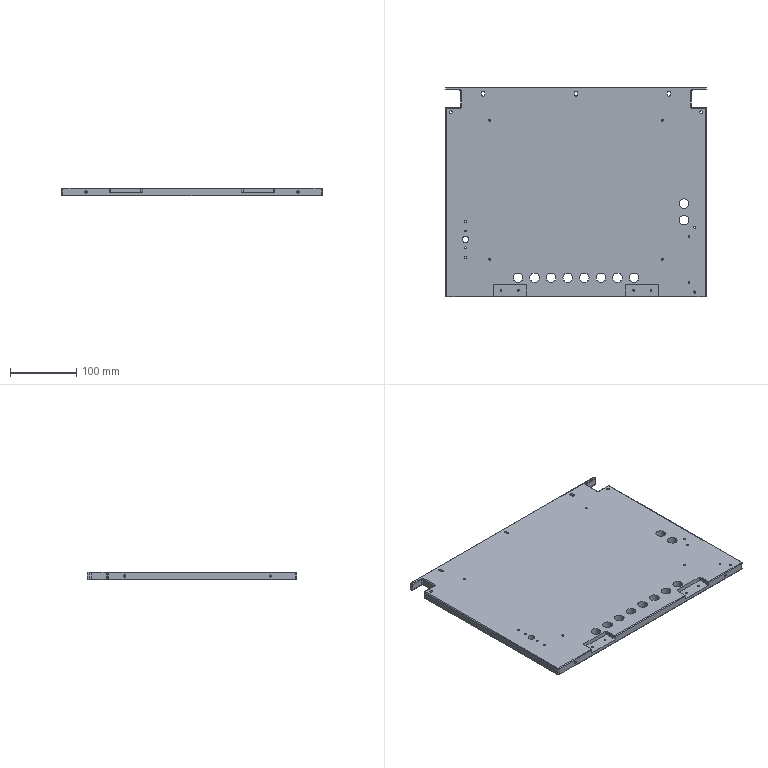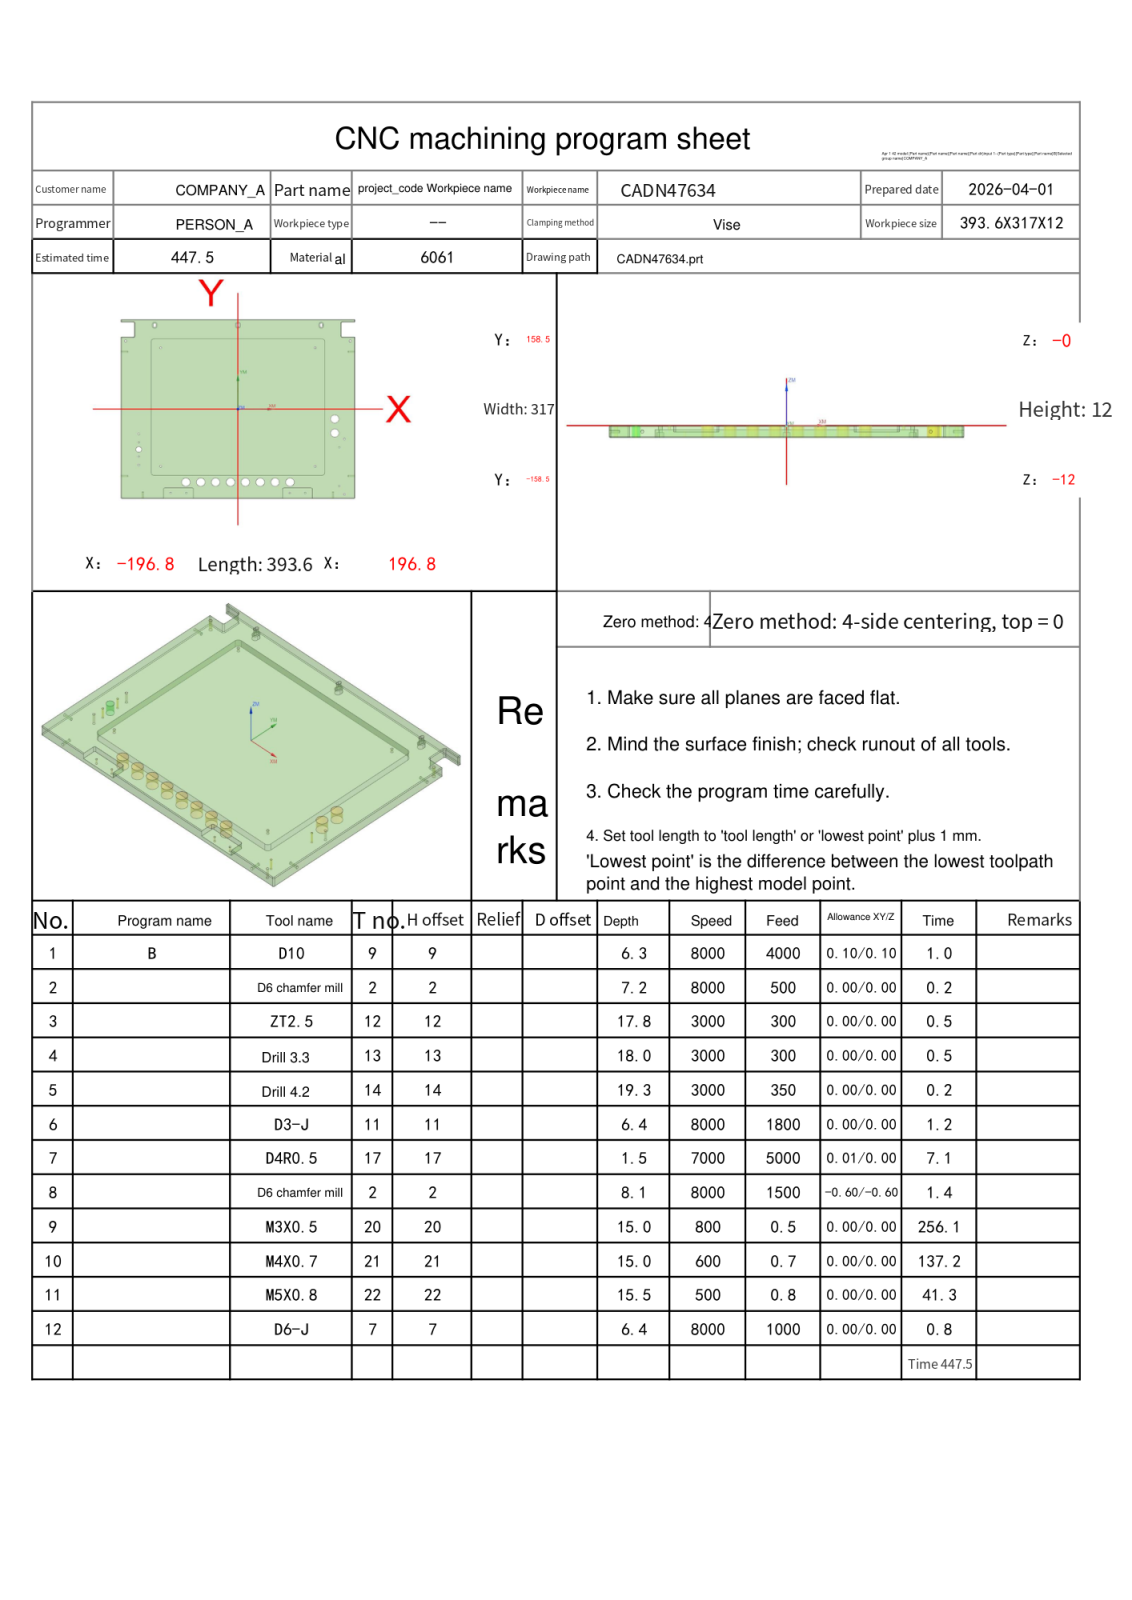NC program | NX | posted by the shop | part box 393.6 x 317 x 12 mm
Lines 710 to 1681 of 6733:
N6 T11 M06
(D3-J  D=3. R=0. H=11 ce=0.00 di=0.00)
G00 G90 G54 X123.199 Y-144.775 M03 S8000
G43 H11 Z20.
M08
Z.151
G01 X123.203 Y-144.774 Z.106 F1800.
X123.214 Y-144.772 Z.064
X123.23 Y-144.767 Z.028
X123.252 Y-144.76 Z-.005
X123.277 Y-144.751 Z-.033
X123.305 Y-144.739 Z-.058
X123.334 Y-144.724 Z-.079
X123.365 Y-144.706 Z-.097
X123.394 Y-144.685 Z-.112
X123.422 Y-144.66 Z-.124
X123.447 Y-144.631 Z-.134
X123.469 Y-144.599 Z-.141
X123.485 Y-144.562 Z-.145
X123.496 Y-144.521 Z-.148
X123.5 Y-144.475 Z-.149
Y-141.5
G03 X123. Y-141. I-.5 J0.0
G01 X120.025
X119.996 Y-141.014
X119.99 Y-141.054 Z-.151
X120.005 Y-141.118 Z-.153
X120.039 Y-141.204 Z-.155
X120.092 Y-141.307 Z-.159
X120.16 Y-141.426 Z-.163
X120.338 Y-141.699 Z-.172
X120.464 Y-141.876 Z-.179
X120.684 Y-142.166 Z-.189
X121.054 Y-142.6 Z-.206
X121.458 Y-143.024 Z-.223
X121.884 Y-143.426 Z-.241
X122.323 Y-143.797 Z-.257
X122.616 Y-144.02 Z-.268
X122.795 Y-144.149 Z-.274
X123.07 Y-144.331 Z-.284
X123.19 Y-144.402 Z-.288
X123.295 Y-144.456 Z-.291
X123.38 Y-144.492 Z-.294
X123.445 Y-144.509 Z-.296
X123.486 Y-144.504 Z-.297
X123.5 Y-144.475 Z-.298
Y-141.5
G03 X123. Y-141. I-.5 J0.0
G01 X120.025
X119.996 Y-141.014
X119.99 Y-141.054 Z-.299
X120.005 Y-141.118 Z-.302
X120.039 Y-141.204 Z-.304
X120.091 Y-141.307 Z-.308
X120.16 Y-141.426 Z-.312
X120.337 Y-141.699 Z-.321
X120.464 Y-141.876 Z-.327
X120.684 Y-142.166 Z-.338
X121.054 Y-142.6 Z-.355
X121.457 Y-143.024 Z-.372
X121.884 Y-143.426 Z-.389
X122.323 Y-143.797 Z-.406
X122.616 Y-144.02 Z-.417
X122.795 Y-144.149 Z-.423
X123.07 Y-144.331 Z-.432
X123.19 Y-144.402 Z-.436
X123.295 Y-144.456 Z-.44
X123.38 Y-144.492 Z-.443
X123.445 Y-144.509 Z-.445
X123.486 Y-144.504 Z-.446
X123.5 Y-144.475 Z-.447
Y-141.5
G03 X123. Y-141. I-.5 J0.0
G01 X120.025
X119.996 Y-141.014
X119.99 Y-141.054 Z-.448
X120.005 Y-141.118 Z-.45
X120.039 Y-141.204 Z-.453
X120.091 Y-141.307 Z-.457
X120.16 Y-141.426 Z-.461
X120.337 Y-141.699 Z-.47
X120.464 Y-141.876 Z-.476
X120.684 Y-142.166 Z-.487
X121.054 Y-142.6 Z-.504
X121.457 Y-143.024 Z-.521
X121.884 Y-143.426 Z-.538
X122.323 Y-143.797 Z-.555
X122.616 Y-144.02 Z-.566
X122.795 Y-144.149 Z-.572
X123.07 Y-144.331 Z-.581
X123.19 Y-144.402 Z-.585
X123.295 Y-144.456 Z-.589
X123.38 Y-144.492 Z-.592
X123.445 Y-144.509 Z-.594
X123.486 Y-144.504 Z-.595
X123.5 Y-144.475
Y-141.5
G03 X123. Y-141. I-.5 J0.0
G01 X120.025
X119.996 Y-141.014 Z-.596
X119.99 Y-141.054 Z-.597
X120.005 Y-141.118 Z-.599
X120.039 Y-141.204 Z-.602
X120.092 Y-141.307 Z-.605
X120.16 Y-141.426 Z-.609
X120.338 Y-141.699 Z-.619
X120.464 Y-141.876 Z-.625
X120.684 Y-142.166 Z-.636
X121.054 Y-142.6 Z-.652
X121.458 Y-143.024 Z-.67
X121.884 Y-143.426 Z-.687
X122.323 Y-143.797 Z-.704
X122.616 Y-144.02 Z-.714
X122.795 Y-144.149 Z-.721
X123.07 Y-144.331 Z-.73
X123.19 Y-144.402 Z-.734
X123.295 Y-144.456 Z-.738
X123.38 Y-144.492 Z-.74
X123.445 Y-144.509 Z-.742
X123.486 Y-144.504 Z-.744
X123.5 Y-144.475
Y-141.5
G03 X123. Y-141. I-.5 J0.0
G01 X120.025
X119.996 Y-141.014 Z-.745
X119.99 Y-141.054 Z-.746
X120.005 Y-141.118 Z-.748
X120.039 Y-141.204 Z-.751
X120.091 Y-141.307 Z-.754
X120.16 Y-141.426 Z-.758
X120.337 Y-141.699 Z-.768
X120.464 Y-141.876 Z-.774
X120.684 Y-142.166 Z-.784
X121.054 Y-142.6 Z-.801
X121.457 Y-143.024 Z-.819
X121.884 Y-143.426 Z-.836
X122.323 Y-143.797 Z-.853
X122.616 Y-144.02 Z-.863
X122.795 Y-144.149 Z-.87
X123.07 Y-144.331 Z-.879
X123.19 Y-144.402 Z-.883
X123.295 Y-144.456 Z-.886
X123.38 Y-144.492 Z-.889
X123.445 Y-144.509 Z-.891
X123.486 Y-144.504 Z-.893
X123.5 Y-144.475
Y-141.5
G03 X123. Y-141. I-.5 J0.0
G01 X120.025
X119.996 Y-141.014
X119.99 Y-141.054 Z-.895
X120.005 Y-141.118 Z-.897
X120.039 Y-141.204 Z-.9
X120.092 Y-141.307 Z-.903
X120.16 Y-141.426 Z-.907
X120.338 Y-141.699 Z-.916
X120.464 Y-141.876 Z-.923
X120.684 Y-142.166 Z-.933
X121.054 Y-142.6 Z-.95
X121.458 Y-143.024 Z-.967
X121.884 Y-143.426 Z-.985
X122.323 Y-143.797 Z-1.002
X122.616 Y-144.02 Z-1.012
X122.795 Y-144.149 Z-1.018
X123.07 Y-144.331 Z-1.028
X123.19 Y-144.402 Z-1.032
X123.295 Y-144.456 Z-1.035
X123.38 Y-144.492 Z-1.038
X123.445 Y-144.509 Z-1.04
X123.486 Y-144.504 Z-1.041
X123.5 Y-144.475 Z-1.042
Y-141.5
G03 X123. Y-141. I-.5 J0.0
G01 X120.025
X119.996 Y-141.014
X119.99 Y-141.054 Z-1.044
X120.005 Y-141.118 Z-1.046
X120.039 Y-141.204 Z-1.048
X120.092 Y-141.307 Z-1.052
X120.16 Y-141.426 Z-1.056
X120.338 Y-141.699 Z-1.065
X120.464 Y-141.876 Z-1.072
X120.684 Y-142.166 Z-1.082
X121.054 Y-142.6 Z-1.099
X121.458 Y-143.024 Z-1.116
X121.884 Y-143.426 Z-1.134
X122.323 Y-143.797 Z-1.15
X122.616 Y-144.02 Z-1.161
X122.795 Y-144.149 Z-1.167
X123.07 Y-144.331 Z-1.177
X123.19 Y-144.402 Z-1.181
X123.295 Y-144.456 Z-1.184
X123.38 Y-144.492 Z-1.187
X123.445 Y-144.509 Z-1.189
X123.486 Y-144.504 Z-1.19
X123.5 Y-144.475 Z-1.191
Y-141.5
G03 X123. Y-141. I-.5 J0.0
G01 X120.025
X119.996 Y-141.014
X119.99 Y-141.054 Z-1.192
X120.005 Y-141.118 Z-1.195
X120.039 Y-141.204 Z-1.197
X120.092 Y-141.307 Z-1.201
X120.16 Y-141.426 Z-1.205
X120.338 Y-141.699 Z-1.214
X120.464 Y-141.876 Z-1.22
X120.684 Y-142.166 Z-1.231
X121.054 Y-142.6 Z-1.248
X121.458 Y-143.024 Z-1.265
X121.884 Y-143.426 Z-1.282
X122.323 Y-143.797 Z-1.299
X122.616 Y-144.02 Z-1.31
X122.795 Y-144.149 Z-1.316
X123.07 Y-144.331 Z-1.325
X123.19 Y-144.402 Z-1.329
X123.295 Y-144.456 Z-1.333
X123.38 Y-144.492 Z-1.336
X123.445 Y-144.509 Z-1.338
X123.486 Y-144.504 Z-1.339
X123.5 Y-144.475 Z-1.34
Y-141.5
G03 X123. Y-141. I-.5 J0.0
G01 X120.025
X119.996 Y-141.014
X119.99 Y-141.054 Z-1.341
X120.005 Y-141.118 Z-1.343
X120.039 Y-141.204 Z-1.346
X120.092 Y-141.307 Z-1.35
X120.16 Y-141.426 Z-1.354
X120.338 Y-141.699 Z-1.363
X120.464 Y-141.876 Z-1.369
X120.684 Y-142.166 Z-1.38
X121.054 Y-142.6 Z-1.397
X121.458 Y-143.024 Z-1.414
X121.884 Y-143.426 Z-1.431
X122.323 Y-143.797 Z-1.448
X122.616 Y-144.02 Z-1.459
X122.795 Y-144.149 Z-1.465
X123.07 Y-144.331 Z-1.474
X123.19 Y-144.402 Z-1.478
X123.295 Y-144.456 Z-1.482
X123.38 Y-144.492 Z-1.485
X123.445 Y-144.509 Z-1.487
X123.486 Y-144.504 Z-1.488
X123.5 Y-144.475
Y-141.5
G03 X123. Y-141. I-.5 J0.0
G01 X120.025
X119.996 Y-141.014 Z-1.489
X119.99 Y-141.054 Z-1.49
X120.005 Y-141.118 Z-1.492
X120.039 Y-141.204 Z-1.495
X120.092 Y-141.307 Z-1.498
X120.16 Y-141.426 Z-1.502
X120.338 Y-141.699 Z-1.512
X120.464 Y-141.876 Z-1.518
X120.684 Y-142.166 Z-1.529
X121.054 Y-142.6 Z-1.545
X121.458 Y-143.024 Z-1.563
X121.884 Y-143.426 Z-1.58
X122.323 Y-143.797 Z-1.597
X122.616 Y-144.02 Z-1.607
X122.795 Y-144.149 Z-1.614
X123.07 Y-144.331 Z-1.623
X123.19 Y-144.402 Z-1.627
X123.295 Y-144.456 Z-1.631
X123.38 Y-144.492 Z-1.633
X123.445 Y-144.509 Z-1.635
X123.486 Y-144.504 Z-1.637
X123.5 Y-144.475
Y-141.5
G03 X123. Y-141. I-.5 J0.0
G01 X120.025
X119.996 Y-141.014 Z-1.638
X119.99 Y-141.054 Z-1.639
X120.005 Y-141.118 Z-1.641
X120.039 Y-141.204 Z-1.644
X120.092 Y-141.307 Z-1.647
X120.16 Y-141.426 Z-1.651
X120.338 Y-141.699 Z-1.661
X120.464 Y-141.876 Z-1.667
X120.684 Y-142.166 Z-1.678
X121.054 Y-142.6 Z-1.694
X121.458 Y-143.024 Z-1.712
X121.884 Y-143.426 Z-1.729
X122.323 Y-143.797 Z-1.746
X122.616 Y-144.02 Z-1.756
X122.795 Y-144.149 Z-1.763
X123.07 Y-144.331 Z-1.772
X123.19 Y-144.402 Z-1.776
X123.295 Y-144.456 Z-1.779
X123.38 Y-144.492 Z-1.782
X123.445 Y-144.509 Z-1.784
X123.486 Y-144.504 Z-1.786
X123.5 Y-144.475
Y-141.5
G03 X123. Y-141. I-.5 J0.0
G01 X120.025
X119.996 Y-141.014
X119.99 Y-141.054 Z-1.788
X120.005 Y-141.118 Z-1.79
X120.039 Y-141.204 Z-1.793
X120.092 Y-141.307 Z-1.796
X120.16 Y-141.426 Z-1.8
X120.338 Y-141.699 Z-1.81
X120.464 Y-141.876 Z-1.816
X120.684 Y-142.166 Z-1.826
X121.054 Y-142.6 Z-1.843
X121.458 Y-143.024 Z-1.86
X121.884 Y-143.426 Z-1.878
X122.323 Y-143.797 Z-1.895
X122.616 Y-144.02 Z-1.905
X122.795 Y-144.149 Z-1.911
X123.07 Y-144.331 Z-1.921
X123.19 Y-144.402 Z-1.925
X123.295 Y-144.456 Z-1.928
X123.38 Y-144.492 Z-1.931
X123.445 Y-144.509 Z-1.933
X123.486 Y-144.504 Z-1.934
X123.5 Y-144.475 Z-1.935
Y-141.5
G03 X123. Y-141. I-.5 J0.0
G01 X120.025
X119.996 Y-141.014
X119.99 Y-141.054 Z-1.937
X120.005 Y-141.118 Z-1.939
X120.039 Y-141.204 Z-1.942
X120.092 Y-141.307 Z-1.945
X120.16 Y-141.426 Z-1.949
X120.338 Y-141.699 Z-1.958
X120.464 Y-141.876 Z-1.965
X120.684 Y-142.166 Z-1.975
X121.054 Y-142.6 Z-1.992
X121.458 Y-143.024 Z-2.009
X121.884 Y-143.426 Z-2.027
X122.323 Y-143.797 Z-2.043
X122.616 Y-144.02 Z-2.054
X122.795 Y-144.149 Z-2.06
X123.07 Y-144.331 Z-2.07
X123.19 Y-144.402 Z-2.074
X123.295 Y-144.456 Z-2.077
X123.38 Y-144.492 Z-2.08
X123.445 Y-144.509 Z-2.082
X123.486 Y-144.504 Z-2.083
X123.5 Y-144.475 Z-2.084
Y-141.5
G03 X123. Y-141. I-.5 J0.0
G01 X120.025
X119.996 Y-141.014
X119.99 Y-141.054 Z-2.085
X120.005 Y-141.118 Z-2.088
X120.039 Y-141.204 Z-2.09
X120.092 Y-141.307 Z-2.094
X120.16 Y-141.426 Z-2.098
X120.338 Y-141.699 Z-2.107
X120.464 Y-141.876 Z-2.113
X120.684 Y-142.166 Z-2.124
X121.054 Y-142.6 Z-2.141
X121.458 Y-143.024 Z-2.158
X121.884 Y-143.426 Z-2.175
X122.323 Y-143.797 Z-2.192
X122.616 Y-144.02 Z-2.203
X122.795 Y-144.149 Z-2.209
X123.07 Y-144.331 Z-2.218
X123.19 Y-144.402 Z-2.222
X123.295 Y-144.456 Z-2.226
X123.38 Y-144.492 Z-2.229
X123.445 Y-144.509 Z-2.231
X123.486 Y-144.504 Z-2.232
X123.5 Y-144.475 Z-2.233
Y-141.5
G03 X123. Y-141. I-.5 J0.0
G01 X120.025
X119.996 Y-141.014
X119.99 Y-141.054 Z-2.234
X120.005 Y-141.118 Z-2.236
X120.039 Y-141.204 Z-2.239
X120.092 Y-141.307 Z-2.243
X120.16 Y-141.426 Z-2.247
X120.338 Y-141.699 Z-2.256
X120.464 Y-141.876 Z-2.262
X120.684 Y-142.166 Z-2.273
X121.054 Y-142.6 Z-2.29
X121.458 Y-143.024 Z-2.307
X121.884 Y-143.426 Z-2.324
X122.323 Y-143.797 Z-2.341
X122.616 Y-144.02 Z-2.352
X122.795 Y-144.149 Z-2.358
X123.07 Y-144.331 Z-2.367
X123.19 Y-144.402 Z-2.371
X123.295 Y-144.456 Z-2.375
X123.38 Y-144.492 Z-2.378
X123.445 Y-144.509 Z-2.38
X123.486 Y-144.504 Z-2.381
X123.5 Y-144.475
Y-141.5
G03 X123. Y-141. I-.5 J0.0
G01 X120.025
X119.996 Y-141.014 Z-2.382
X119.99 Y-141.054 Z-2.383
X120.005 Y-141.118 Z-2.385
X120.039 Y-141.204 Z-2.388
X120.092 Y-141.307 Z-2.391
X120.16 Y-141.426 Z-2.395
X120.338 Y-141.699 Z-2.405
X120.464 Y-141.876 Z-2.411
X120.684 Y-142.166 Z-2.422
X121.054 Y-142.6 Z-2.438
X121.458 Y-143.024 Z-2.456
X121.884 Y-143.426 Z-2.473
X122.323 Y-143.797 Z-2.49
X122.616 Y-144.02 Z-2.5
X122.795 Y-144.149 Z-2.507
X123.07 Y-144.331 Z-2.516
X123.19 Y-144.402 Z-2.52
X123.295 Y-144.456 Z-2.524
X123.38 Y-144.492 Z-2.526
X123.445 Y-144.509 Z-2.528
X123.486 Y-144.504 Z-2.53
X123.5 Y-144.475
Y-141.5
G03 X123. Y-141. I-.5 J0.0
G01 X120.025
X119.996 Y-141.014 Z-2.531
X119.99 Y-141.054 Z-2.532
X120.005 Y-141.118 Z-2.534
X120.039 Y-141.204 Z-2.537
X120.092 Y-141.307 Z-2.54
X120.16 Y-141.426 Z-2.544
X120.338 Y-141.699 Z-2.554
X120.464 Y-141.876 Z-2.56
X120.684 Y-142.166 Z-2.571
X121.054 Y-142.6 Z-2.587
X121.458 Y-143.024 Z-2.605
X121.884 Y-143.426 Z-2.622
X122.323 Y-143.797 Z-2.639
X122.616 Y-144.02 Z-2.649
X122.795 Y-144.149 Z-2.656
X123.07 Y-144.331 Z-2.665
X123.19 Y-144.402 Z-2.669
X123.295 Y-144.456 Z-2.672
X123.38 Y-144.492 Z-2.675
X123.445 Y-144.509 Z-2.677
X123.486 Y-144.504 Z-2.679
X123.5 Y-144.475
Y-141.5
G03 X123. Y-141. I-.5 J0.0
G01 X120.025
X119.996 Y-141.014 Z-2.68
X119.99 Y-141.054 Z-2.681
X120.005 Y-141.118 Z-2.683
X120.039 Y-141.204 Z-2.686
X120.092 Y-141.307 Z-2.689
X120.16 Y-141.426 Z-2.693
X120.338 Y-141.699 Z-2.703
X120.464 Y-141.876 Z-2.709
X120.684 Y-142.166 Z-2.719
X121.054 Y-142.6 Z-2.736
X121.458 Y-143.024 Z-2.753
X121.884 Y-143.426 Z-2.771
X122.323 Y-143.797 Z-2.788
X122.616 Y-144.02 Z-2.798
X122.795 Y-144.149 Z-2.804
X123.07 Y-144.331 Z-2.814
X123.19 Y-144.402 Z-2.818
X123.295 Y-144.456 Z-2.821
X123.38 Y-144.492 Z-2.824
X123.445 Y-144.509 Z-2.826
X123.486 Y-144.504 Z-2.827
X123.5 Y-144.475 Z-2.828
Y-141.5
G03 X123. Y-141. I-.5 J0.0
G01 X120.025
X119.996 Y-141.014
X119.99 Y-141.054 Z-2.83
X120.005 Y-141.118 Z-2.832
X120.039 Y-141.204 Z-2.835
X120.092 Y-141.307 Z-2.838
X120.16 Y-141.426 Z-2.842
X120.338 Y-141.699 Z-2.851
X120.464 Y-141.876 Z-2.858
X120.684 Y-142.166 Z-2.868
X121.054 Y-142.6 Z-2.885
X121.458 Y-143.024 Z-2.902
X121.884 Y-143.426 Z-2.92
X122.323 Y-143.797 Z-2.936
X122.616 Y-144.02 Z-2.947
X122.795 Y-144.149 Z-2.953
X123.07 Y-144.331 Z-2.963
X123.19 Y-144.402 Z-2.967
X123.295 Y-144.456 Z-2.97
X123.38 Y-144.492 Z-2.973
X123.445 Y-144.509 Z-2.975
X123.486 Y-144.504 Z-2.976
X123.5 Y-144.475 Z-2.977
Y-141.5
G03 X123. Y-141. I-.5 J0.0
G01 X120.025
X119.996 Y-141.014
X119.99 Y-141.054 Z-2.978
X120.005 Y-141.118 Z-2.981
X120.039 Y-141.204 Z-2.983
X120.092 Y-141.307 Z-2.987
X120.16 Y-141.426 Z-2.991
X120.338 Y-141.699 Z-3.
X120.464 Y-141.876 Z-3.007
X120.684 Y-142.166 Z-3.017
X121.054 Y-142.6 Z-3.034
X121.458 Y-143.024 Z-3.051
X121.884 Y-143.426 Z-3.069
X122.323 Y-143.797 Z-3.085
X122.616 Y-144.02 Z-3.096
X122.795 Y-144.149 Z-3.102
X123.07 Y-144.331 Z-3.111
X123.19 Y-144.402 Z-3.116
X123.295 Y-144.456 Z-3.119
X123.38 Y-144.492 Z-3.122
X123.445 Y-144.509 Z-3.124
X123.486 Y-144.504 Z-3.125
X123.5 Y-144.475 Z-3.126
Y-141.5
G03 X123. Y-141. I-.5 J0.0
G01 X120.025
X119.996 Y-141.014
X119.99 Y-141.054 Z-3.127
X120.005 Y-141.118 Z-3.129
X120.039 Y-141.204 Z-3.132
X120.092 Y-141.307 Z-3.136
X120.16 Y-141.426 Z-3.14
X120.338 Y-141.699 Z-3.149
X120.464 Y-141.876 Z-3.155
X120.684 Y-142.166 Z-3.166
X121.054 Y-142.6 Z-3.183
X121.458 Y-143.024 Z-3.2
X121.884 Y-143.426 Z-3.217
X122.323 Y-143.797 Z-3.234
X122.616 Y-144.02 Z-3.245
X122.795 Y-144.149 Z-3.251
X123.07 Y-144.331 Z-3.26
X123.19 Y-144.402 Z-3.264
X123.295 Y-144.456 Z-3.268
X123.38 Y-144.492 Z-3.271
X123.445 Y-144.509 Z-3.273
X123.486 Y-144.504 Z-3.274
X123.5 Y-144.475
Y-141.5
G03 X123. Y-141. I-.5 J0.0
G01 X120.025
X119.996 Y-141.014 Z-3.275
X119.99 Y-141.054 Z-3.276
X120.005 Y-141.118 Z-3.278
X120.039 Y-141.204 Z-3.281
X120.092 Y-141.307 Z-3.284
X120.16 Y-141.426 Z-3.289
X120.338 Y-141.699 Z-3.298
X120.464 Y-141.876 Z-3.304
X120.684 Y-142.166 Z-3.315
X121.054 Y-142.6 Z-3.331
X121.458 Y-143.024 Z-3.349
X121.884 Y-143.426 Z-3.366
X122.323 Y-143.797 Z-3.383
X122.616 Y-144.02 Z-3.394
X122.795 Y-144.149 Z-3.4
X123.07 Y-144.331 Z-3.409
X123.19 Y-144.402 Z-3.413
X123.295 Y-144.456 Z-3.417
X123.38 Y-144.492 Z-3.419
X123.445 Y-144.509 Z-3.422
X123.486 Y-144.504 Z-3.423
X123.5 Y-144.475
Y-141.5
G03 X123. Y-141. I-.5 J0.0
G01 X120.025
X119.996 Y-141.014 Z-3.424
X119.99 Y-141.054 Z-3.425
X120.005 Y-141.118 Z-3.427
X120.039 Y-141.204 Z-3.43
X120.092 Y-141.307 Z-3.433
X120.16 Y-141.426 Z-3.437
X120.338 Y-141.699 Z-3.447
X120.464 Y-141.876 Z-3.453
X120.684 Y-142.166 Z-3.464
X121.054 Y-142.6 Z-3.48
X121.458 Y-143.024 Z-3.498
X121.884 Y-143.426 Z-3.515
X122.323 Y-143.797 Z-3.532
X122.616 Y-144.02 Z-3.542
X122.795 Y-144.149 Z-3.549
X123.07 Y-144.331 Z-3.558
X123.19 Y-144.402 Z-3.562
X123.295 Y-144.456 Z-3.565
X123.38 Y-144.492 Z-3.568
X123.445 Y-144.509 Z-3.57
X123.486 Y-144.504 Z-3.572
X123.5 Y-144.475
Y-141.5
G03 X123. Y-141. I-.5 J0.0
G01 X120.025
X119.996 Y-141.014 Z-3.573
X119.99 Y-141.054 Z-3.574
X120.005 Y-141.118 Z-3.576
X120.039 Y-141.204 Z-3.579
X120.092 Y-141.307 Z-3.582
X120.16 Y-141.426 Z-3.586
X120.338 Y-141.699 Z-3.596
X120.464 Y-141.876 Z-3.602
X120.684 Y-142.166 Z-3.612
X121.054 Y-142.6 Z-3.629
X121.458 Y-143.024 Z-3.647
X121.884 Y-143.426 Z-3.664
X122.323 Y-143.797 Z-3.681
X122.616 Y-144.02 Z-3.691
X122.795 Y-144.149 Z-3.697
X123.07 Y-144.331 Z-3.707
X123.19 Y-144.402 Z-3.711
X123.295 Y-144.456 Z-3.714
X123.38 Y-144.492 Z-3.717
X123.445 Y-144.509 Z-3.719
X123.486 Y-144.504 Z-3.72
X123.5 Y-144.475 Z-3.721
Y-141.5
G03 X123. Y-141. I-.5 J0.0
G01 X120.025
X119.996 Y-141.014
X119.99 Y-141.054 Z-3.723
X120.005 Y-141.118 Z-3.725
X120.039 Y-141.204 Z-3.728
X120.092 Y-141.307 Z-3.731
X120.16 Y-141.426 Z-3.735
X120.338 Y-141.699 Z-3.744
X120.464 Y-141.876 Z-3.751
X120.684 Y-142.166 Z-3.761
X121.054 Y-142.6 Z-3.778
X121.458 Y-143.024 Z-3.795
X121.884 Y-143.426 Z-3.813
X122.323 Y-143.797 Z-3.829
X122.616 Y-144.02 Z-3.84
X122.795 Y-144.149 Z-3.846
X123.07 Y-144.331 Z-3.856
X123.19 Y-144.402 Z-3.86
X123.295 Y-144.456 Z-3.863
X123.38 Y-144.492 Z-3.866
X123.445 Y-144.509 Z-3.868
X123.486 Y-144.504 Z-3.869
X123.5 Y-144.475 Z-3.87
Y-141.5
G03 X123. Y-141. I-.5 J0.0
G01 X120.025
X119.996 Y-141.014
X119.99 Y-141.054 Z-3.872
X120.005 Y-141.118 Z-3.874
X120.039 Y-141.204 Z-3.876
X120.092 Y-141.307 Z-3.88
X120.16 Y-141.426 Z-3.884
X120.338 Y-141.699 Z-3.893
X120.464 Y-141.876 Z-3.9
X120.684 Y-142.166 Z-3.91
X121.054 Y-142.6 Z-3.927
X121.458 Y-143.024 Z-3.944
X121.884 Y-143.426 Z-3.962
X122.323 Y-143.797 Z-3.978
X122.616 Y-144.02 Z-3.989
X122.795 Y-144.149 Z-3.995
X123.07 Y-144.331 Z-4.005
X123.19 Y-144.402 Z-4.009
X123.295 Y-144.456 Z-4.012
X123.38 Y-144.492 Z-4.015
X123.445 Y-144.509 Z-4.017
X123.486 Y-144.504 Z-4.018
X123.5 Y-144.475 Z-4.019
Y-141.5
G03 X123. Y-141. I-.5 J0.0
G01 X120.025
X119.996 Y-141.014
X119.99 Y-141.054 Z-4.02
X120.005 Y-141.118 Z-4.022
X120.039 Y-141.204 Z-4.025
X120.092 Y-141.307 Z-4.029
X120.16 Y-141.426 Z-4.033
X120.338 Y-141.699 Z-4.042
X120.464 Y-141.876 Z-4.048
X120.684 Y-142.166 Z-4.059
X121.054 Y-142.6 Z-4.076
X121.458 Y-143.024 Z-4.093
X121.884 Y-143.426 Z-4.11
X122.323 Y-143.797 Z-4.127
X122.616 Y-144.02 Z-4.138
X122.795 Y-144.149 Z-4.144
X123.07 Y-144.331 Z-4.153
X123.19 Y-144.402 Z-4.157
X123.295 Y-144.456 Z-4.161
X123.38 Y-144.492 Z-4.164
X123.445 Y-144.509 Z-4.166
X123.486 Y-144.504 Z-4.167
X123.5 Y-144.475
Y-141.5
G03 X123. Y-141. I-.5 J0.0
G01 X120.025
X119.996 Y-141.014 Z-4.168
X119.99 Y-141.054 Z-4.169
X120.005 Y-141.118 Z-4.171
X120.039 Y-141.204 Z-4.174
X120.092 Y-141.307 Z-4.178
X120.16 Y-141.426 Z-4.182
X120.338 Y-141.699 Z-4.191
X120.464 Y-141.876 Z-4.197
X120.684 Y-142.166 Z-4.208
X121.054 Y-142.6 Z-4.225
X121.458 Y-143.024 Z-4.242
X121.884 Y-143.426 Z-4.259
X122.323 Y-143.797 Z-4.276
X122.616 Y-144.02 Z-4.287
X122.795 Y-144.149 Z-4.293
X123.07 Y-144.331 Z-4.302
X123.19 Y-144.402 Z-4.306
X123.295 Y-144.456 Z-4.31
X123.38 Y-144.492 Z-4.312
X123.445 Y-144.509 Z-4.315
X123.486 Y-144.504 Z-4.316
X123.5 Y-144.475
Y-141.5
G03 X123. Y-141. I-.5 J0.0
G01 X120.025
X119.996 Y-141.014 Z-4.317
X119.99 Y-141.054 Z-4.318
X120.005 Y-141.118 Z-4.32
X120.039 Y-141.204 Z-4.323
X120.092 Y-141.307 Z-4.326
X120.16 Y-141.426 Z-4.33
X120.338 Y-141.699 Z-4.34
X120.464 Y-141.876 Z-4.346
X120.684 Y-142.166 Z-4.357
X121.054 Y-142.6 Z-4.373
X121.458 Y-143.024 Z-4.391
X121.884 Y-143.426 Z-4.408
X122.323 Y-143.797 Z-4.425
X122.616 Y-144.02 Z-4.435
X122.795 Y-144.149 Z-4.442
X123.07 Y-144.331 Z-4.451
X123.19 Y-144.402 Z-4.455
X123.295 Y-144.456 Z-4.458
X123.38 Y-144.492 Z-4.461
X123.445 Y-144.509 Z-4.463
X123.486 Y-144.504 Z-4.465
X123.5 Y-144.475
Y-141.5
G03 X123. Y-141. I-.5 J0.0
G01 X120.025
X119.996 Y-141.014 Z-4.466
X119.99 Y-141.054 Z-4.467
X120.005 Y-141.118 Z-4.469
X120.039 Y-141.204 Z-4.472
X120.092 Y-141.307 Z-4.475
X120.16 Y-141.426 Z-4.479
X120.338 Y-141.699 Z-4.489
X120.464 Y-141.876 Z-4.495
X120.684 Y-142.166 Z-4.505
X121.054 Y-142.6 Z-4.522
X121.458 Y-143.024 Z-4.54
X121.884 Y-143.426 Z-4.557
X122.323 Y-143.797 Z-4.574
X122.616 Y-144.02 Z-4.584
X122.795 Y-144.149 Z-4.59
X123.07 Y-144.331 Z-4.6
X123.19 Y-144.402 Z-4.604
X123.295 Y-144.456 Z-4.607
X123.38 Y-144.492 Z-4.61
X123.445 Y-144.509 Z-4.612
X123.486 Y-144.504 Z-4.614
X123.5 Y-144.475
Y-141.5
G03 X123. Y-141. I-.5 J0.0
G01 X120.025
X119.996 Y-141.014
X119.99 Y-141.054 Z-4.616
X120.005 Y-141.118 Z-4.618
X120.039 Y-141.204 Z-4.621
X120.092 Y-141.307 Z-4.624
X120.16 Y-141.426 Z-4.628
X120.338 Y-141.699 Z-4.637
X120.464 Y-141.876 Z-4.644
X120.684 Y-142.166 Z-4.654
X121.054 Y-142.6 Z-4.671
X121.458 Y-143.024 Z-4.688
X121.884 Y-143.426 Z-4.706
X122.323 Y-143.797 Z-4.722
X122.616 Y-144.02 Z-4.733
X122.795 Y-144.149 Z-4.739
X123.07 Y-144.331 Z-4.749
X123.19 Y-144.402 Z-4.753
X123.295 Y-144.456 Z-4.756
X123.38 Y-144.492 Z-4.759
X123.445 Y-144.509 Z-4.761
X123.486 Y-144.504 Z-4.762
X123.5 Y-144.475 Z-4.763
Y-141.5
G03 X123. Y-141. I-.5 J0.0
G01 X120.025
X119.996 Y-141.014
X119.99 Y-141.054 Z-4.765
X120.005 Y-141.118 Z-4.767
X120.039 Y-141.204 Z-4.769
X120.092 Y-141.307 Z-4.773
X120.16 Y-141.426 Z-4.777
X120.338 Y-141.699 Z-4.786
X120.464 Y-141.876 Z-4.793
X120.684 Y-142.166 Z-4.803
X121.054 Y-142.6 Z-4.82
X121.458 Y-143.024 Z-4.837
X121.884 Y-143.426 Z-4.855
X122.323 Y-143.797 Z-4.871
X122.616 Y-144.02 Z-4.882
X122.795 Y-144.149 Z-4.888
X123.07 Y-144.331 Z-4.898
X123.19 Y-144.402 Z-4.902
X123.295 Y-144.456 Z-4.905
X123.38 Y-144.492 Z-4.908
X123.445 Y-144.509 Z-4.91
X123.486 Y-144.504 Z-4.911
X123.5 Y-144.475 Z-4.912
Y-141.5
G03 X123. Y-141. I-.5 J0.0
G01 X120.025
X119.996 Y-141.014
X119.99 Y-141.054 Z-4.913
X120.005 Y-141.118 Z-4.915
X120.039 Y-141.204 Z-4.918
X120.092 Y-141.307 Z-4.922
X120.16 Y-141.426 Z-4.926
X120.338 Y-141.699 Z-4.935
X120.464 Y-141.876 Z-4.941
X120.684 Y-142.166 Z-4.952
X121.054 Y-142.6 Z-4.969
X121.458 Y-143.024 Z-4.986
X121.884 Y-143.426 Z-5.003
X122.323 Y-143.797 Z-5.02
X122.616 Y-144.02 Z-5.031
X122.795 Y-144.149 Z-5.037
X123.07 Y-144.331 Z-5.046
X123.19 Y-144.402 Z-5.05
X123.295 Y-144.456 Z-5.054
X123.38 Y-144.492 Z-5.057
X123.445 Y-144.509 Z-5.059
X123.486 Y-144.504 Z-5.06
X123.5 Y-144.475
Y-141.5
G03 X123. Y-141. I-.5 J0.0
G01 X120.025
X119.996 Y-141.014 Z-5.061
X119.99 Y-141.054 Z-5.062
X120.005 Y-141.118 Z-5.064
X120.039 Y-141.204 Z-5.067
X120.092 Y-141.307 Z-5.071
X120.16 Y-141.426 Z-5.075
X120.338 Y-141.699 Z-5.084
X120.464 Y-141.876 Z-5.09
X120.684 Y-142.166 Z-5.101
X121.054 Y-142.6 Z-5.118
X121.458 Y-143.024 Z-5.135
X121.884 Y-143.426 Z-5.152
X122.323 Y-143.797 Z-5.169
X122.616 Y-144.02 Z-5.18
X122.795 Y-144.149 Z-5.186
X123.07 Y-144.331 Z-5.195
X123.19 Y-144.402 Z-5.199
X123.295 Y-144.456 Z-5.203
X123.38 Y-144.492 Z-5.205
X123.445 Y-144.509 Z-5.208
X123.486 Y-144.504 Z-5.209
X123.5 Y-144.475
Y-141.5
G03 X123. Y-141. I-.5 J0.0
G01 X120.025
X119.996 Y-141.014 Z-5.21
X119.99 Y-141.054 Z-5.211
X120.005 Y-141.118 Z-5.213
X120.039 Y-141.204 Z-5.216
X120.092 Y-141.307 Z-5.219
X120.16 Y-141.426 Z-5.223
X120.338 Y-141.699 Z-5.233
X120.464 Y-141.876 Z-5.239
X120.684 Y-142.166 Z-5.25
X121.054 Y-142.6 Z-5.266
X121.458 Y-143.024 Z-5.284
X121.884 Y-143.426 Z-5.301
X122.323 Y-143.797 Z-5.318
X122.616 Y-144.02 Z-5.328
X122.795 Y-144.149 Z-5.335
X123.07 Y-144.331 Z-5.344
X123.19 Y-144.402 Z-5.348
X123.295 Y-144.456 Z-5.352
X123.38 Y-144.492 Z-5.354
X123.445 Y-144.509 Z-5.356
X123.486 Y-144.504 Z-5.358
X123.5 Y-144.475
Y-141.5
G03 X123. Y-141. I-.5 J0.0
G01 X120.025
X119.996 Y-141.014 Z-5.359
X119.99 Y-141.054 Z-5.36
X120.005 Y-141.118 Z-5.362
X120.039 Y-141.204 Z-5.365
X120.092 Y-141.307 Z-5.368
X120.16 Y-141.426 Z-5.372
X120.338 Y-141.699 Z-5.382
X120.464 Y-141.876 Z-5.388
X120.684 Y-142.166 Z-5.398
X121.054 Y-142.6 Z-5.415
X121.458 Y-143.024 Z-5.433
X121.884 Y-143.426 Z-5.45
X122.323 Y-143.797 Z-5.467
X122.616 Y-144.02 Z-5.477
X122.795 Y-144.149 Z-5.484
X123.07 Y-144.331 Z-5.493
X123.19 Y-144.402 Z-5.497
X123.295 Y-144.456 Z-5.5
X123.38 Y-144.492 Z-5.503
X123.445 Y-144.509 Z-5.505
X123.486 Y-144.504 Z-5.507
X123.5 Y-144.475
Y-141.5
G03 X123. Y-141. I-.5 J0.0
G01 X120.025
X119.996 Y-141.014
X119.99 Y-141.054 Z-5.509
X120.005 Y-141.118 Z-5.511
X120.039 Y-141.204 Z-5.514
X120.092 Y-141.307 Z-5.517
X120.16 Y-141.426 Z-5.521
X120.338 Y-141.699 Z-5.53
X120.464 Y-141.876 Z-5.537
X120.684 Y-142.166 Z-5.547
X121.054 Y-142.6 Z-5.564
X121.458 Y-143.024 Z-5.581
X121.884 Y-143.426 Z-5.599
X122.323 Y-143.797 Z-5.616
X122.616 Y-144.02 Z-5.626
X122.795 Y-144.149 Z-5.632
X123.07 Y-144.331 Z-5.642
X123.19 Y-144.402 Z-5.646
X123.295 Y-144.456 Z-5.649
X123.38 Y-144.492 Z-5.652
X123.445 Y-144.509 Z-5.654
X123.486 Y-144.504 Z-5.655
X123.5 Y-144.475 Z-5.656
Y-141.5
G03 X123. Y-141. I-.5 J0.0
G01 X120.025
X119.996 Y-141.014
X119.99 Y-141.054 Z-5.658
X120.005 Y-141.118 Z-5.66
X120.039 Y-141.204 Z-5.662
X120.092 Y-141.307 Z-5.666
X120.16 Y-141.426 Z-5.67
X120.338 Y-141.699 Z-5.679
X120.464 Y-141.876 Z-5.686
X120.684 Y-142.166 Z-5.696
X121.054 Y-142.6 Z-5.713
X121.458 Y-143.024 Z-5.73
X121.884 Y-143.426 Z-5.748
X122.323 Y-143.797 Z-5.764
X122.616 Y-144.02 Z-5.775
X122.795 Y-144.149 Z-5.781
X123.07 Y-144.331 Z-5.791
X123.19 Y-144.402 Z-5.795
X123.295 Y-144.456 Z-5.798
X123.38 Y-144.492 Z-5.801
X123.445 Y-144.509 Z-5.803
X123.486 Y-144.504 Z-5.804
X123.5 Y-144.475 Z-5.805
Y-141.5